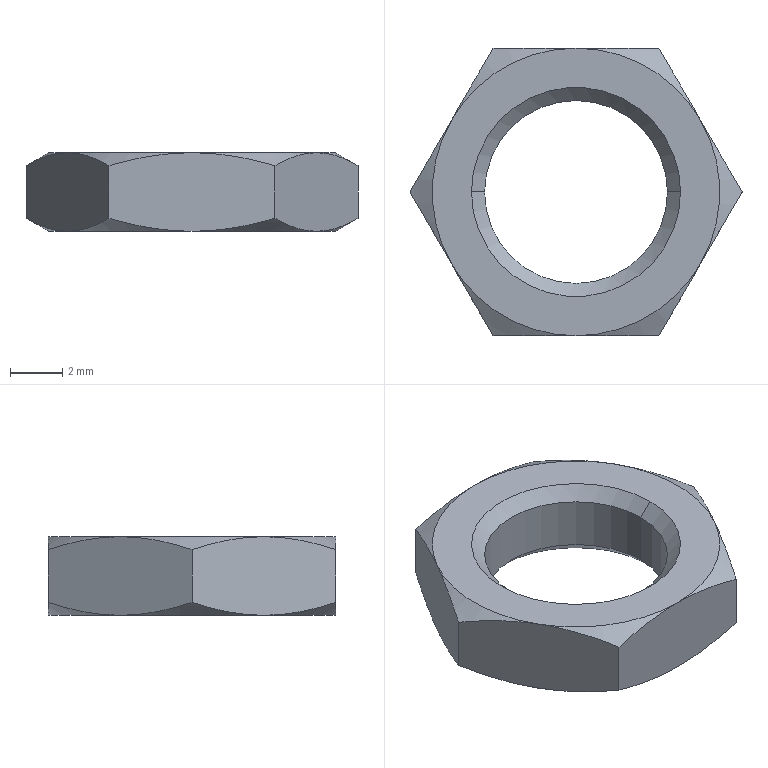Part | STEP file | QA-SKSC0806-2 | 1 solid | 27 faces | box 12.702 x 11 x 3 mm | volume 190.264 mm3 | cone 17 | plane 8 | cylinder 2 | commonest cylinder face diameters 7 x2